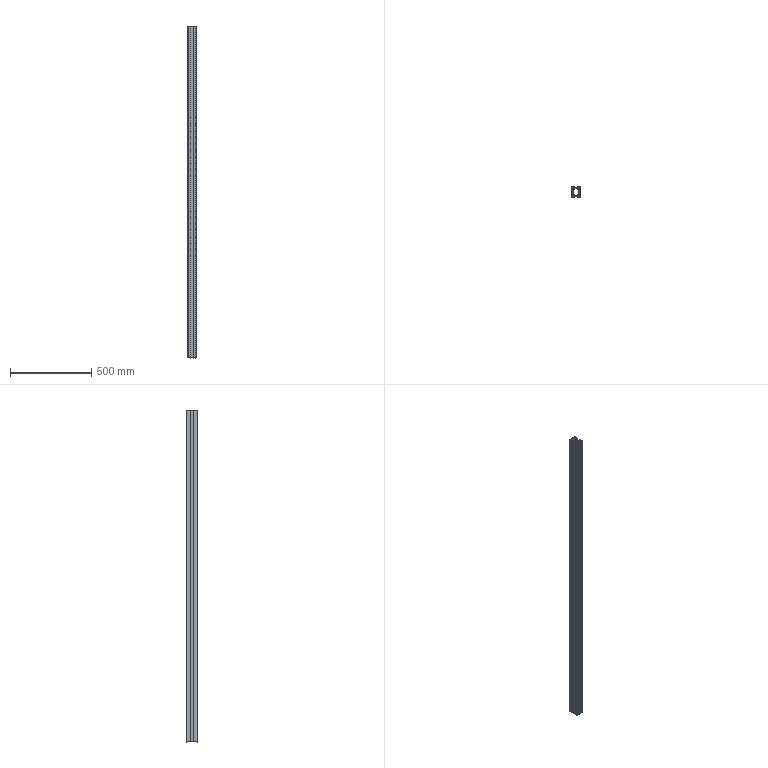Part | STEP file | 46A-00010CC11-2040mm | 1 solid | 143 faces | box 50 x 70 x 2040 mm | volume 1443284 mm3 | cylinder 85 | plane 58 | commonest cylinder face diameters 1 x25 4 x24 1.5 x16 3.7 x8 6.7 x8 2 x4